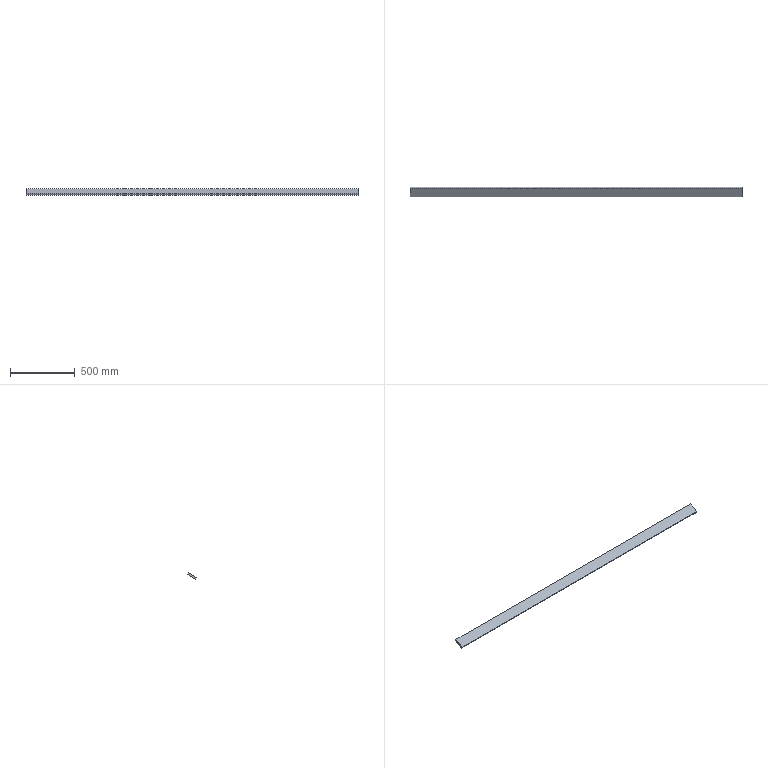Part | NX | features 底座(默认<按焊接>) 2 | 1 solid | 6 faces | box 2570 x 74.293 x 53.683 mm | volume 3173441 mm3 | plane 6
STEP:
#1=CARTESIAN_POINT('',(2531.685,87.82,-918.));
#2=VERTEX_POINT('',#1);
#3=CARTESIAN_POINT('',(2531.685,96.113,-931.683));
#4=VERTEX_POINT('',#3);
#5=CARTESIAN_POINT('',(2531.685,96.113,-931.683));
#6=DIRECTION('',(0.,0.5183,-0.8552));
#7=VECTOR('',#6,1000.);
#8=LINE('',#5,#7);
#9=EDGE_CURVE('',#2,#4,#8,.T.);
#10=ORIENTED_EDGE('',*,*,#9,.T.);
#11=CARTESIAN_POINT('',(-38.315,96.113,-931.683));
#12=VERTEX_POINT('',#11);
#13=CARTESIAN_POINT('',(-38.315,96.113,-931.683));
#14=DIRECTION('',(1.,0.,0.));
#15=VECTOR('',#14,1000.);
#16=LINE('',#13,#15);
#17=EDGE_CURVE('',#12,#4,#16,.T.);
#18=ORIENTED_EDGE('',*,*,#17,.F.);
#19=CARTESIAN_POINT('',(-38.315,87.82,-918.));
#20=VERTEX_POINT('',#19);
#21=CARTESIAN_POINT('',(-38.315,96.113,-931.683));
#22=DIRECTION('',(0.,0.5183,-0.8552));
#23=VECTOR('',#22,1000.);
#24=LINE('',#21,#23);
#25=EDGE_CURVE('',#20,#12,#24,.T.);
#26=ORIENTED_EDGE('',*,*,#25,.F.);
#27=CARTESIAN_POINT('',(-38.315,87.82,-918.));
#28=DIRECTION('',(1.,0.,0.));
#29=VECTOR('',#28,1000.);
#30=LINE('',#27,#29);
#31=EDGE_CURVE('',#20,#2,#30,.T.);
#32=ORIENTED_EDGE('',*,*,#31,.T.);
#33=EDGE_LOOP('',(#10,#18,#26,#32));
#34=FACE_BOUND('',#33,.T.);
#35=CARTESIAN_POINT('',(-38.315,96.113,-931.683));
#36=DIRECTION('',(0.,0.8552,0.5183));
#37=DIRECTION('',(0.,0.5183,-0.8552));
#38=AXIS2_PLACEMENT_3D('',#35,#36,#37);
#39=PLANE('',#38);
#40=ADVANCED_FACE('',(#34),#39,.T.);
#41=CARTESIAN_POINT('',(2531.685,21.82,-958.));
#42=VERTEX_POINT('',#41);
#43=CARTESIAN_POINT('',(2531.685,87.82,-918.));
#44=DIRECTION('',(0.,0.8552,0.5183));
#45=VECTOR('',#44,1000.);
#46=LINE('',#43,#45);
#47=EDGE_CURVE('',#42,#2,#46,.T.);
#48=ORIENTED_EDGE('',*,*,#47,.T.);
#49=ORIENTED_EDGE('',*,*,#31,.F.);
#50=CARTESIAN_POINT('',(-38.315,21.82,-958.));
#51=VERTEX_POINT('',#50);
#52=CARTESIAN_POINT('',(-38.315,87.82,-918.));
#53=DIRECTION('',(0.,0.8552,0.5183));
#54=VECTOR('',#53,1000.);
#55=LINE('',#52,#54);
#56=EDGE_CURVE('',#51,#20,#55,.T.);
#57=ORIENTED_EDGE('',*,*,#56,.F.);
#58=CARTESIAN_POINT('',(-38.315,21.82,-958.));
#59=DIRECTION('',(1.,0.,0.));
#60=VECTOR('',#59,1000.);
#61=LINE('',#58,#60);
#62=EDGE_CURVE('',#51,#42,#61,.T.);
#63=ORIENTED_EDGE('',*,*,#62,.T.);
#64=EDGE_LOOP('',(#48,#49,#57,#63));
#65=FACE_BOUND('',#64,.T.);
#66=CARTESIAN_POINT('',(-38.315,87.82,-918.));
#67=DIRECTION('',(0.,-0.5183,0.8552));
#68=DIRECTION('',(0.,0.8552,0.5183));
#69=AXIS2_PLACEMENT_3D('',#66,#67,#68);
#70=PLANE('',#69);
#71=ADVANCED_FACE('',(#65),#70,.T.);
#72=CARTESIAN_POINT('',(2531.685,30.113,-971.683));
#73=VERTEX_POINT('',#72);
#74=CARTESIAN_POINT('',(2531.685,30.113,-971.683));
#75=DIRECTION('',(0.,-0.5183,0.8552));
#76=VECTOR('',#75,1000.);
#77=LINE('',#74,#76);
#78=EDGE_CURVE('',#73,#42,#77,.T.);
#79=ORIENTED_EDGE('',*,*,#78,.T.);
#80=ORIENTED_EDGE('',*,*,#62,.F.);
#81=CARTESIAN_POINT('',(-38.315,30.113,-971.683));
#82=VERTEX_POINT('',#81);
#83=CARTESIAN_POINT('',(-38.315,30.113,-971.683));
#84=DIRECTION('',(0.,-0.5183,0.8552));
#85=VECTOR('',#84,1000.);
#86=LINE('',#83,#85);
#87=EDGE_CURVE('',#82,#51,#86,.T.);
#88=ORIENTED_EDGE('',*,*,#87,.F.);
#89=CARTESIAN_POINT('',(-38.315,30.113,-971.683));
#90=DIRECTION('',(1.,0.,0.));
#91=VECTOR('',#90,1000.);
#92=LINE('',#89,#91);
#93=EDGE_CURVE('',#82,#73,#92,.T.);
#94=ORIENTED_EDGE('',*,*,#93,.T.);
#95=EDGE_LOOP('',(#79,#80,#88,#94));
#96=FACE_BOUND('',#95,.T.);
#97=CARTESIAN_POINT('',(-38.315,30.113,-971.683));
#98=DIRECTION('',(0.,-0.8552,-0.5183));
#99=DIRECTION('',(0.,-0.5183,0.8552));
#100=AXIS2_PLACEMENT_3D('',#97,#98,#99);
#101=PLANE('',#100);
#102=ADVANCED_FACE('',(#96),#101,.T.);
#103=CARTESIAN_POINT('',(2531.685,96.113,-931.683));
#104=DIRECTION('',(0.,-0.8552,-0.5183));
#105=VECTOR('',#104,1000.);
#106=LINE('',#103,#105);
#107=EDGE_CURVE('',#4,#73,#106,.T.);
#108=ORIENTED_EDGE('',*,*,#107,.T.);
#109=ORIENTED_EDGE('',*,*,#93,.F.);
#110=CARTESIAN_POINT('',(-38.315,96.113,-931.683));
#111=DIRECTION('',(0.,-0.8552,-0.5183));
#112=VECTOR('',#111,1000.);
#113=LINE('',#110,#112);
#114=EDGE_CURVE('',#12,#82,#113,.T.);
#115=ORIENTED_EDGE('',*,*,#114,.F.);
#116=ORIENTED_EDGE('',*,*,#17,.T.);
#117=EDGE_LOOP('',(#108,#109,#115,#116));
#118=FACE_BOUND('',#117,.T.);
#119=CARTESIAN_POINT('',(-38.315,96.113,-931.683));
#120=DIRECTION('',(0.,0.5183,-0.8552));
#121=DIRECTION('',(0.,-0.8552,-0.5183));
#122=AXIS2_PLACEMENT_3D('',#119,#120,#121);
#123=PLANE('',#122);
#124=ADVANCED_FACE('',(#118),#123,.T.);
#125=ORIENTED_EDGE('',*,*,#25,.T.);
#126=ORIENTED_EDGE('',*,*,#114,.T.);
#127=ORIENTED_EDGE('',*,*,#87,.T.);
#128=ORIENTED_EDGE('',*,*,#56,.T.);
#129=EDGE_LOOP('',(#125,#126,#127,#128));
#130=FACE_BOUND('',#129,.T.);
#131=CARTESIAN_POINT('',(-38.315,87.82,-918.));
#132=DIRECTION('',(-1.,0.,0.));
#133=DIRECTION('',(0.,0.,-1.));
#134=AXIS2_PLACEMENT_3D('',#131,#132,#133);
#135=PLANE('',#134);
#136=ADVANCED_FACE('',(#130),#135,.T.);
#137=ORIENTED_EDGE('',*,*,#9,.F.);
#138=ORIENTED_EDGE('',*,*,#47,.F.);
#139=ORIENTED_EDGE('',*,*,#78,.F.);
#140=ORIENTED_EDGE('',*,*,#107,.F.);
#141=EDGE_LOOP('',(#137,#138,#139,#140));
#142=FACE_BOUND('',#141,.T.);
#143=CARTESIAN_POINT('',(2531.685,87.82,-918.));
#144=DIRECTION('',(-1.,0.,0.));
#145=DIRECTION('',(0.,0.,-1.));
#146=AXIS2_PLACEMENT_3D('',#143,#144,#145);
#147=PLANE('',#146);
#148=ADVANCED_FACE('',(#142),#147,.F.);
#149=CLOSED_SHELL('',(#40,#71,#102,#124,#136,#148));
#150=MANIFOLD_SOLID_BREP('',#149);
#151=(LENGTH_UNIT()NAMED_UNIT(*)SI_UNIT(.MILLI.,.METRE.));
#152=UNCERTAINTY_MEASURE_WITH_UNIT(LENGTH_MEASURE(0.00001),#151,'','');
#153=(NAMED_UNIT(*)PLANE_ANGLE_UNIT()SI_UNIT($,.RADIAN.));
#154=(NAMED_UNIT(*)SI_UNIT($,.STERADIAN.)SOLID_ANGLE_UNIT());
#155=(GEOMETRIC_REPRESENTATION_CONTEXT(3)GLOBAL_UNCERTAINTY_ASSIGNED_CONTEXT((#152))GLOBAL_UNIT_ASSIGNED_CONTEXT((#151,#153,#154))REPRESENTATION_CONTEXT('',''));
#156=ADVANCED_BREP_SHAPE_REPRESENTATION('',(#150),#155);